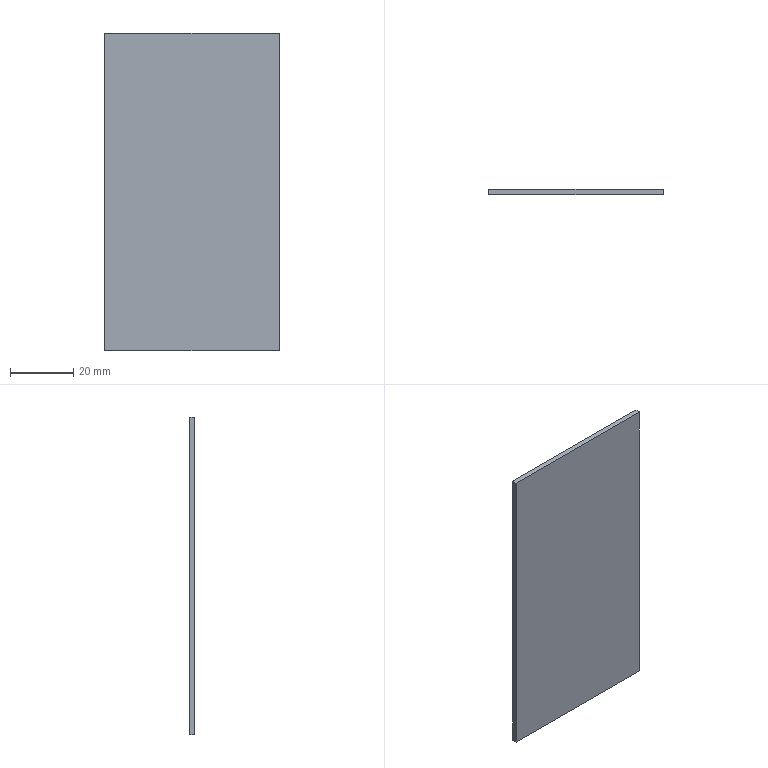Part | STEP file | 1 solid | 6 faces | box 55 x 1.5 x 100 mm | volume 8250 mm3 | plane 6
STEP:
#1=CARTESIAN_POINT('',(0.,0.,0.));
#2=DIRECTION('',(0.,0.,1.));
#3=DIRECTION('',(1.,0.,0.));
#4=AXIS2_PLACEMENT_3D('',#1,#2,#3);
#5=CARTESIAN_POINT('',(27.5,0.,50.));
#6=VERTEX_POINT('',#5);
#7=CARTESIAN_POINT('',(27.5,0.,-50.));
#8=VERTEX_POINT('',#7);
#9=CARTESIAN_POINT('',(27.5,0.,-50.));
#10=DIRECTION('',(0.,0.,-1.));
#11=VECTOR('',#10,1.);
#12=LINE('',#9,#11);
#13=CARTESIAN_POINT('',(27.5,1.5,-50.));
#14=DIRECTION('',(-1.,0.,0.));
#15=DIRECTION('',(0.,0.,1.));
#16=AXIS2_PLACEMENT_3D('',#13,#14,#15);
#17=PLANE('',#16);
#18=CARTESIAN_POINT('',(0.,-1.5));
#19=DIRECTION('',(-1.,0.));
#20=VECTOR('',#19,1.);
#21=LINE('',#18,#20);
#22=(GEOMETRIC_REPRESENTATION_CONTEXT(2)PARAMETRIC_REPRESENTATION_CONTEXT()REPRESENTATION_CONTEXT('',''));
#23=DEFINITIONAL_REPRESENTATION('',(#21),#22);
#24=PCURVE('',#17,#23);
#25=CARTESIAN_POINT('',(0.,0.,0.));
#26=DIRECTION('',(0.,1.,0.));
#27=DIRECTION('',(0.,0.,1.));
#28=AXIS2_PLACEMENT_3D('',#25,#26,#27);
#29=PLANE('',#28);
#30=CARTESIAN_POINT('',(-50.,27.5));
#31=DIRECTION('',(-1.,0.));
#32=VECTOR('',#31,1.);
#33=LINE('',#30,#32);
#34=(GEOMETRIC_REPRESENTATION_CONTEXT(2)PARAMETRIC_REPRESENTATION_CONTEXT()REPRESENTATION_CONTEXT('',''));
#35=DEFINITIONAL_REPRESENTATION('',(#33),#34);
#36=PCURVE('',#29,#35);
#37=SURFACE_CURVE('',#12,(#24,#36),.PCURVE_S1.);
#38=EDGE_CURVE('',#6,#8,#37,.T.);
#39=ORIENTED_EDGE('',*,*,#38,.T.);
#40=CARTESIAN_POINT('',(27.5,1.5,-50.));
#41=VERTEX_POINT('',#40);
#42=CARTESIAN_POINT('',(27.5,1.5,-50.));
#43=DIRECTION('',(0.,-1.,0.));
#44=VECTOR('',#43,1.);
#45=LINE('',#42,#44);
#46=CARTESIAN_POINT('',(0.,0.));
#47=DIRECTION('',(0.,-1.));
#48=VECTOR('',#47,1.);
#49=LINE('',#46,#48);
#50=(GEOMETRIC_REPRESENTATION_CONTEXT(2)PARAMETRIC_REPRESENTATION_CONTEXT()REPRESENTATION_CONTEXT('',''));
#51=DEFINITIONAL_REPRESENTATION('',(#49),#50);
#52=PCURVE('',#17,#51);
#53=CARTESIAN_POINT('',(-27.5,1.5,-50.));
#54=DIRECTION('',(0.,0.,1.));
#55=DIRECTION('',(1.,0.,0.));
#56=AXIS2_PLACEMENT_3D('',#53,#54,#55);
#57=PLANE('',#56);
#58=CARTESIAN_POINT('',(55.,0.));
#59=DIRECTION('',(0.,-1.));
#60=VECTOR('',#59,1.);
#61=LINE('',#58,#60);
#62=(GEOMETRIC_REPRESENTATION_CONTEXT(2)PARAMETRIC_REPRESENTATION_CONTEXT()REPRESENTATION_CONTEXT('',''));
#63=DEFINITIONAL_REPRESENTATION('',(#61),#62);
#64=PCURVE('',#57,#63);
#65=SURFACE_CURVE('',#45,(#52,#64),.PCURVE_S1.);
#66=EDGE_CURVE('',#41,#8,#65,.T.);
#67=ORIENTED_EDGE('',*,*,#66,.F.);
#68=CARTESIAN_POINT('',(27.5,1.5,50.));
#69=VERTEX_POINT('',#68);
#70=CARTESIAN_POINT('',(27.5,1.5,-50.));
#71=DIRECTION('',(0.,0.,-1.));
#72=VECTOR('',#71,1.);
#73=LINE('',#70,#72);
#74=CARTESIAN_POINT('',(0.,0.));
#75=DIRECTION('',(-1.,0.));
#76=VECTOR('',#75,1.);
#77=LINE('',#74,#76);
#78=(GEOMETRIC_REPRESENTATION_CONTEXT(2)PARAMETRIC_REPRESENTATION_CONTEXT()REPRESENTATION_CONTEXT('',''));
#79=DEFINITIONAL_REPRESENTATION('',(#77),#78);
#80=PCURVE('',#17,#79);
#81=CARTESIAN_POINT('',(0.,1.5,0.));
#82=DIRECTION('',(0.,1.,0.));
#83=DIRECTION('',(0.,0.,1.));
#84=AXIS2_PLACEMENT_3D('',#81,#82,#83);
#85=PLANE('',#84);
#86=CARTESIAN_POINT('',(-50.,27.5));
#87=DIRECTION('',(-1.,0.));
#88=VECTOR('',#87,1.);
#89=LINE('',#86,#88);
#90=(GEOMETRIC_REPRESENTATION_CONTEXT(2)PARAMETRIC_REPRESENTATION_CONTEXT()REPRESENTATION_CONTEXT('',''));
#91=DEFINITIONAL_REPRESENTATION('',(#89),#90);
#92=PCURVE('',#85,#91);
#93=SURFACE_CURVE('',#73,(#80,#92),.PCURVE_S1.);
#94=EDGE_CURVE('',#69,#41,#93,.T.);
#95=ORIENTED_EDGE('',*,*,#94,.F.);
#96=CARTESIAN_POINT('',(27.5,1.5,50.));
#97=DIRECTION('',(0.,-1.,0.));
#98=VECTOR('',#97,1.);
#99=LINE('',#96,#98);
#100=CARTESIAN_POINT('',(100.,0.));
#101=DIRECTION('',(0.,-1.));
#102=VECTOR('',#101,1.);
#103=LINE('',#100,#102);
#104=(GEOMETRIC_REPRESENTATION_CONTEXT(2)PARAMETRIC_REPRESENTATION_CONTEXT()REPRESENTATION_CONTEXT('',''));
#105=DEFINITIONAL_REPRESENTATION('',(#103),#104);
#106=PCURVE('',#17,#105);
#107=CARTESIAN_POINT('',(-27.5,1.5,50.));
#108=DIRECTION('',(0.,0.,-1.));
#109=DIRECTION('',(-1.,0.,0.));
#110=AXIS2_PLACEMENT_3D('',#107,#108,#109);
#111=PLANE('',#110);
#112=CARTESIAN_POINT('',(-55.,0.));
#113=DIRECTION('',(0.,-1.));
#114=VECTOR('',#113,1.);
#115=LINE('',#112,#114);
#116=(GEOMETRIC_REPRESENTATION_CONTEXT(2)PARAMETRIC_REPRESENTATION_CONTEXT()REPRESENTATION_CONTEXT('',''));
#117=DEFINITIONAL_REPRESENTATION('',(#115),#116);
#118=PCURVE('',#111,#117);
#119=SURFACE_CURVE('',#99,(#106,#118),.PCURVE_S1.);
#120=EDGE_CURVE('',#69,#6,#119,.T.);
#121=ORIENTED_EDGE('',*,*,#120,.T.);
#122=EDGE_LOOP('',(#39,#67,#95,#121));
#123=FACE_BOUND('',#122,.T.);
#124=ADVANCED_FACE('',(#123),#17,.F.);
#125=CARTESIAN_POINT('',(-27.5,0.,-50.));
#126=VERTEX_POINT('',#125);
#127=CARTESIAN_POINT('',(-27.5,0.,-50.));
#128=DIRECTION('',(-1.,0.,0.));
#129=VECTOR('',#128,1.);
#130=LINE('',#127,#129);
#131=CARTESIAN_POINT('',(0.,-1.5));
#132=DIRECTION('',(-1.,0.));
#133=VECTOR('',#132,1.);
#134=LINE('',#131,#133);
#135=(GEOMETRIC_REPRESENTATION_CONTEXT(2)PARAMETRIC_REPRESENTATION_CONTEXT()REPRESENTATION_CONTEXT('',''));
#136=DEFINITIONAL_REPRESENTATION('',(#134),#135);
#137=PCURVE('',#57,#136);
#138=CARTESIAN_POINT('',(-50.,-27.5));
#139=DIRECTION('',(0.,-1.));
#140=VECTOR('',#139,1.);
#141=LINE('',#138,#140);
#142=(GEOMETRIC_REPRESENTATION_CONTEXT(2)PARAMETRIC_REPRESENTATION_CONTEXT()REPRESENTATION_CONTEXT('',''));
#143=DEFINITIONAL_REPRESENTATION('',(#141),#142);
#144=PCURVE('',#29,#143);
#145=SURFACE_CURVE('',#130,(#137,#144),.PCURVE_S1.);
#146=EDGE_CURVE('',#8,#126,#145,.T.);
#147=ORIENTED_EDGE('',*,*,#146,.T.);
#148=CARTESIAN_POINT('',(-27.5,1.5,-50.));
#149=VERTEX_POINT('',#148);
#150=CARTESIAN_POINT('',(-27.5,1.5,-50.));
#151=DIRECTION('',(0.,-1.,0.));
#152=VECTOR('',#151,1.);
#153=LINE('',#150,#152);
#154=CARTESIAN_POINT('',(0.,0.));
#155=DIRECTION('',(0.,-1.));
#156=VECTOR('',#155,1.);
#157=LINE('',#154,#156);
#158=(GEOMETRIC_REPRESENTATION_CONTEXT(2)PARAMETRIC_REPRESENTATION_CONTEXT()REPRESENTATION_CONTEXT('',''));
#159=DEFINITIONAL_REPRESENTATION('',(#157),#158);
#160=PCURVE('',#57,#159);
#161=CARTESIAN_POINT('',(-27.5,1.5,-50.));
#162=DIRECTION('',(1.,0.,0.));
#163=DIRECTION('',(0.,0.,-1.));
#164=AXIS2_PLACEMENT_3D('',#161,#162,#163);
#165=PLANE('',#164);
#166=CARTESIAN_POINT('',(0.,0.));
#167=DIRECTION('',(0.,-1.));
#168=VECTOR('',#167,1.);
#169=LINE('',#166,#168);
#170=(GEOMETRIC_REPRESENTATION_CONTEXT(2)PARAMETRIC_REPRESENTATION_CONTEXT()REPRESENTATION_CONTEXT('',''));
#171=DEFINITIONAL_REPRESENTATION('',(#169),#170);
#172=PCURVE('',#165,#171);
#173=SURFACE_CURVE('',#153,(#160,#172),.PCURVE_S1.);
#174=EDGE_CURVE('',#149,#126,#173,.T.);
#175=ORIENTED_EDGE('',*,*,#174,.F.);
#176=CARTESIAN_POINT('',(-27.5,1.5,-50.));
#177=DIRECTION('',(-1.,0.,0.));
#178=VECTOR('',#177,1.);
#179=LINE('',#176,#178);
#180=CARTESIAN_POINT('',(0.,0.));
#181=DIRECTION('',(-1.,0.));
#182=VECTOR('',#181,1.);
#183=LINE('',#180,#182);
#184=(GEOMETRIC_REPRESENTATION_CONTEXT(2)PARAMETRIC_REPRESENTATION_CONTEXT()REPRESENTATION_CONTEXT('',''));
#185=DEFINITIONAL_REPRESENTATION('',(#183),#184);
#186=PCURVE('',#57,#185);
#187=CARTESIAN_POINT('',(-50.,-27.5));
#188=DIRECTION('',(0.,-1.));
#189=VECTOR('',#188,1.);
#190=LINE('',#187,#189);
#191=(GEOMETRIC_REPRESENTATION_CONTEXT(2)PARAMETRIC_REPRESENTATION_CONTEXT()REPRESENTATION_CONTEXT('',''));
#192=DEFINITIONAL_REPRESENTATION('',(#190),#191);
#193=PCURVE('',#85,#192);
#194=SURFACE_CURVE('',#179,(#186,#193),.PCURVE_S1.);
#195=EDGE_CURVE('',#41,#149,#194,.T.);
#196=ORIENTED_EDGE('',*,*,#195,.F.);
#197=ORIENTED_EDGE('',*,*,#66,.T.);
#198=EDGE_LOOP('',(#147,#175,#196,#197));
#199=FACE_BOUND('',#198,.T.);
#200=ADVANCED_FACE('',(#199),#57,.F.);
#201=CARTESIAN_POINT('',(-27.5,0.,50.));
#202=VERTEX_POINT('',#201);
#203=CARTESIAN_POINT('',(-27.5,0.,-50.));
#204=DIRECTION('',(0.,0.,1.));
#205=VECTOR('',#204,1.);
#206=LINE('',#203,#205);
#207=CARTESIAN_POINT('',(0.,-1.5));
#208=DIRECTION('',(-1.,0.));
#209=VECTOR('',#208,1.);
#210=LINE('',#207,#209);
#211=(GEOMETRIC_REPRESENTATION_CONTEXT(2)PARAMETRIC_REPRESENTATION_CONTEXT()REPRESENTATION_CONTEXT('',''));
#212=DEFINITIONAL_REPRESENTATION('',(#210),#211);
#213=PCURVE('',#165,#212);
#214=CARTESIAN_POINT('',(-50.,-27.5));
#215=DIRECTION('',(1.,0.));
#216=VECTOR('',#215,1.);
#217=LINE('',#214,#216);
#218=(GEOMETRIC_REPRESENTATION_CONTEXT(2)PARAMETRIC_REPRESENTATION_CONTEXT()REPRESENTATION_CONTEXT('',''));
#219=DEFINITIONAL_REPRESENTATION('',(#217),#218);
#220=PCURVE('',#29,#219);
#221=SURFACE_CURVE('',#206,(#213,#220),.PCURVE_S1.);
#222=EDGE_CURVE('',#126,#202,#221,.T.);
#223=ORIENTED_EDGE('',*,*,#222,.T.);
#224=CARTESIAN_POINT('',(-27.5,1.5,50.));
#225=VERTEX_POINT('',#224);
#226=CARTESIAN_POINT('',(-27.5,1.5,50.));
#227=DIRECTION('',(0.,-1.,0.));
#228=VECTOR('',#227,1.);
#229=LINE('',#226,#228);
#230=CARTESIAN_POINT('',(-100.,0.));
#231=DIRECTION('',(0.,-1.));
#232=VECTOR('',#231,1.);
#233=LINE('',#230,#232);
#234=(GEOMETRIC_REPRESENTATION_CONTEXT(2)PARAMETRIC_REPRESENTATION_CONTEXT()REPRESENTATION_CONTEXT('',''));
#235=DEFINITIONAL_REPRESENTATION('',(#233),#234);
#236=PCURVE('',#165,#235);
#237=CARTESIAN_POINT('',(0.,0.));
#238=DIRECTION('',(0.,-1.));
#239=VECTOR('',#238,1.);
#240=LINE('',#237,#239);
#241=(GEOMETRIC_REPRESENTATION_CONTEXT(2)PARAMETRIC_REPRESENTATION_CONTEXT()REPRESENTATION_CONTEXT('',''));
#242=DEFINITIONAL_REPRESENTATION('',(#240),#241);
#243=PCURVE('',#111,#242);
#244=SURFACE_CURVE('',#229,(#236,#243),.PCURVE_S1.);
#245=EDGE_CURVE('',#225,#202,#244,.T.);
#246=ORIENTED_EDGE('',*,*,#245,.F.);
#247=CARTESIAN_POINT('',(-27.5,1.5,-50.));
#248=DIRECTION('',(0.,0.,1.));
#249=VECTOR('',#248,1.);
#250=LINE('',#247,#249);
#251=CARTESIAN_POINT('',(0.,0.));
#252=DIRECTION('',(-1.,0.));
#253=VECTOR('',#252,1.);
#254=LINE('',#251,#253);
#255=(GEOMETRIC_REPRESENTATION_CONTEXT(2)PARAMETRIC_REPRESENTATION_CONTEXT()REPRESENTATION_CONTEXT('',''));
#256=DEFINITIONAL_REPRESENTATION('',(#254),#255);
#257=PCURVE('',#165,#256);
#258=CARTESIAN_POINT('',(-50.,-27.5));
#259=DIRECTION('',(1.,0.));
#260=VECTOR('',#259,1.);
#261=LINE('',#258,#260);
#262=(GEOMETRIC_REPRESENTATION_CONTEXT(2)PARAMETRIC_REPRESENTATION_CONTEXT()REPRESENTATION_CONTEXT('',''));
#263=DEFINITIONAL_REPRESENTATION('',(#261),#262);
#264=PCURVE('',#85,#263);
#265=SURFACE_CURVE('',#250,(#257,#264),.PCURVE_S1.);
#266=EDGE_CURVE('',#149,#225,#265,.T.);
#267=ORIENTED_EDGE('',*,*,#266,.F.);
#268=ORIENTED_EDGE('',*,*,#174,.T.);
#269=EDGE_LOOP('',(#223,#246,#267,#268));
#270=FACE_BOUND('',#269,.T.);
#271=ADVANCED_FACE('',(#270),#165,.F.);
#272=CARTESIAN_POINT('',(-27.5,0.,50.));
#273=DIRECTION('',(1.,0.,0.));
#274=VECTOR('',#273,1.);
#275=LINE('',#272,#274);
#276=CARTESIAN_POINT('',(0.,-1.5));
#277=DIRECTION('',(-1.,0.));
#278=VECTOR('',#277,1.);
#279=LINE('',#276,#278);
#280=(GEOMETRIC_REPRESENTATION_CONTEXT(2)PARAMETRIC_REPRESENTATION_CONTEXT()REPRESENTATION_CONTEXT('',''));
#281=DEFINITIONAL_REPRESENTATION('',(#279),#280);
#282=PCURVE('',#111,#281);
#283=CARTESIAN_POINT('',(50.,-27.5));
#284=DIRECTION('',(0.,1.));
#285=VECTOR('',#284,1.);
#286=LINE('',#283,#285);
#287=(GEOMETRIC_REPRESENTATION_CONTEXT(2)PARAMETRIC_REPRESENTATION_CONTEXT()REPRESENTATION_CONTEXT('',''));
#288=DEFINITIONAL_REPRESENTATION('',(#286),#287);
#289=PCURVE('',#29,#288);
#290=SURFACE_CURVE('',#275,(#282,#289),.PCURVE_S1.);
#291=EDGE_CURVE('',#202,#6,#290,.T.);
#292=ORIENTED_EDGE('',*,*,#291,.T.);
#293=ORIENTED_EDGE('',*,*,#120,.F.);
#294=CARTESIAN_POINT('',(-27.5,1.5,50.));
#295=DIRECTION('',(1.,0.,0.));
#296=VECTOR('',#295,1.);
#297=LINE('',#294,#296);
#298=CARTESIAN_POINT('',(0.,0.));
#299=DIRECTION('',(-1.,0.));
#300=VECTOR('',#299,1.);
#301=LINE('',#298,#300);
#302=(GEOMETRIC_REPRESENTATION_CONTEXT(2)PARAMETRIC_REPRESENTATION_CONTEXT()REPRESENTATION_CONTEXT('',''));
#303=DEFINITIONAL_REPRESENTATION('',(#301),#302);
#304=PCURVE('',#111,#303);
#305=CARTESIAN_POINT('',(50.,-27.5));
#306=DIRECTION('',(0.,1.));
#307=VECTOR('',#306,1.);
#308=LINE('',#305,#307);
#309=(GEOMETRIC_REPRESENTATION_CONTEXT(2)PARAMETRIC_REPRESENTATION_CONTEXT()REPRESENTATION_CONTEXT('',''));
#310=DEFINITIONAL_REPRESENTATION('',(#308),#309);
#311=PCURVE('',#85,#310);
#312=SURFACE_CURVE('',#297,(#304,#311),.PCURVE_S1.);
#313=EDGE_CURVE('',#225,#69,#312,.T.);
#314=ORIENTED_EDGE('',*,*,#313,.F.);
#315=ORIENTED_EDGE('',*,*,#245,.T.);
#316=EDGE_LOOP('',(#292,#293,#314,#315));
#317=FACE_BOUND('',#316,.T.);
#318=ADVANCED_FACE('',(#317),#111,.F.);
#319=ORIENTED_EDGE('',*,*,#94,.T.);
#320=ORIENTED_EDGE('',*,*,#195,.T.);
#321=ORIENTED_EDGE('',*,*,#266,.T.);
#322=ORIENTED_EDGE('',*,*,#313,.T.);
#323=EDGE_LOOP('',(#319,#320,#321,#322));
#324=FACE_BOUND('',#323,.T.);
#325=ADVANCED_FACE('',(#324),#85,.T.);
#326=ORIENTED_EDGE('',*,*,#38,.F.);
#327=ORIENTED_EDGE('',*,*,#291,.F.);
#328=ORIENTED_EDGE('',*,*,#222,.F.);
#329=ORIENTED_EDGE('',*,*,#146,.F.);
#330=EDGE_LOOP('',(#326,#327,#328,#329));
#331=FACE_BOUND('',#330,.T.);
#332=ADVANCED_FACE('',(#331),#29,.F.);
#333=CLOSED_SHELL('',(#124,#200,#271,#318,#325,#332));
#334=MANIFOLD_SOLID_BREP('',#333);
#335=(LENGTH_UNIT()NAMED_UNIT(*)SI_UNIT(.MILLI.,.METRE.));
#336=UNCERTAINTY_MEASURE_WITH_UNIT(LENGTH_MEASURE(0.0000001),#335,'','');
#337=(NAMED_UNIT(*)PLANE_ANGLE_UNIT()SI_UNIT($,.RADIAN.));
#338=(NAMED_UNIT(*)SI_UNIT($,.STERADIAN.)SOLID_ANGLE_UNIT());
#339=(GEOMETRIC_REPRESENTATION_CONTEXT(3)GLOBAL_UNCERTAINTY_ASSIGNED_CONTEXT((#336))GLOBAL_UNIT_ASSIGNED_CONTEXT((#335,#337,#338))REPRESENTATION_CONTEXT('',''));
#340=ADVANCED_BREP_SHAPE_REPRESENTATION('',(#4,#334),#339);